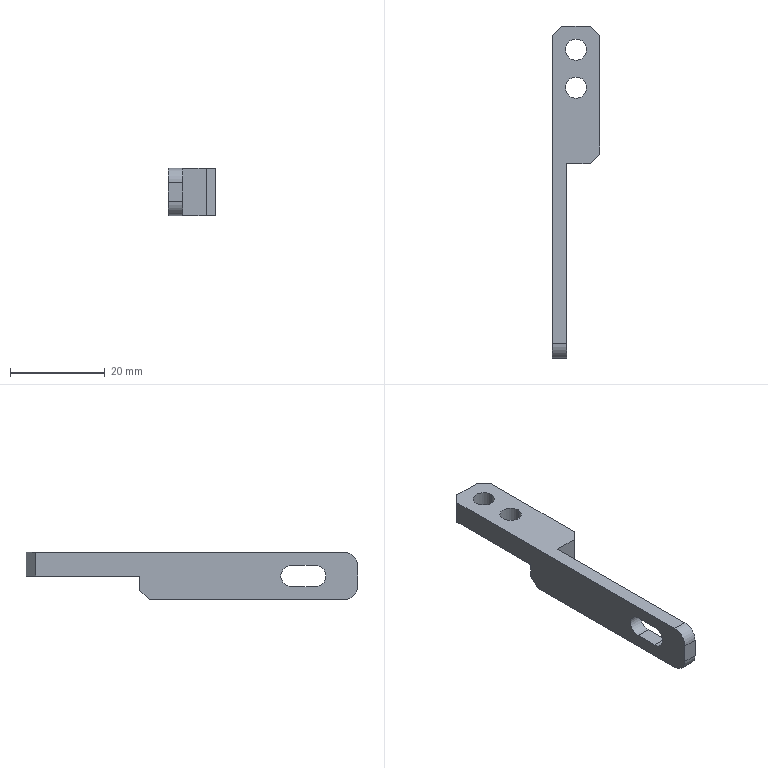Part | SolidWorks | features ICE 3, Chamfer 1, Extrusion 1, Fillet 1, HoleWzd 1 | 1 solid | 24 faces | box 10 x 70 x 10 mm | volume 2584 mm3 | plane 16 | cylinder 8 | commonest cylinder face diameters 4.5 x6 6 x2
STEP:
#1=CARTESIAN_POINT('',(-2.25,30.,0.));
#2=VERTEX_POINT('',#1);
#3=CARTESIAN_POINT('',(2.25,30.,0.));
#4=VERTEX_POINT('',#3);
#5=CARTESIAN_POINT('',(0.,30.,0.));
#6=DIRECTION('',(0.,0.,1.));
#7=DIRECTION('',(0.,-1.,0.));
#8=AXIS2_PLACEMENT_3D('',#5,#6,#7);
#9=CIRCLE('',#8,2.25);
#10=EDGE_CURVE('',#2,#4,#9,.T.);
#11=ORIENTED_EDGE('',*,*,#10,.F.);
#12=CARTESIAN_POINT('',(-2.25,30.,5.));
#13=VERTEX_POINT('',#12);
#14=CARTESIAN_POINT('',(-2.25,30.,5.));
#15=DIRECTION('',(0.,0.,1.));
#16=VECTOR('',#15,1000.);
#17=LINE('',#14,#16);
#18=EDGE_CURVE('',#2,#13,#17,.T.);
#19=ORIENTED_EDGE('',*,*,#18,.T.);
#20=CARTESIAN_POINT('',(2.25,30.,5.));
#21=VERTEX_POINT('',#20);
#22=CARTESIAN_POINT('',(0.,30.,5.));
#23=DIRECTION('',(0.,0.,1.));
#24=DIRECTION('',(1.,0.,0.));
#25=AXIS2_PLACEMENT_3D('',#22,#23,#24);
#26=CIRCLE('',#25,2.25);
#27=EDGE_CURVE('',#13,#21,#26,.T.);
#28=ORIENTED_EDGE('',*,*,#27,.T.);
#29=CARTESIAN_POINT('',(2.25,30.,5.));
#30=DIRECTION('',(0.,0.,1.));
#31=VECTOR('',#30,1000.);
#32=LINE('',#29,#31);
#33=EDGE_CURVE('',#4,#21,#32,.T.);
#34=ORIENTED_EDGE('',*,*,#33,.F.);
#35=EDGE_LOOP('',(#11,#19,#28,#34));
#36=FACE_OUTER_BOUND('',#35,.T.);
#37=CARTESIAN_POINT('',(0.,30.,5.));
#38=DIRECTION('',(0.,0.,1.));
#39=DIRECTION('',(1.,0.,0.));
#40=AXIS2_PLACEMENT_3D('',#37,#38,#39);
#41=CYLINDRICAL_SURFACE('',#40,2.25);
#42=ADVANCED_FACE('',(#36),#41,.F.);
#43=CARTESIAN_POINT('',(-2.25,22.,0.));
#44=VERTEX_POINT('',#43);
#45=CARTESIAN_POINT('',(2.25,22.,0.));
#46=VERTEX_POINT('',#45);
#47=CARTESIAN_POINT('',(0.,22.,0.));
#48=DIRECTION('',(0.,0.,1.));
#49=DIRECTION('',(0.,-1.,0.));
#50=AXIS2_PLACEMENT_3D('',#47,#48,#49);
#51=CIRCLE('',#50,2.25);
#52=EDGE_CURVE('',#44,#46,#51,.T.);
#53=ORIENTED_EDGE('',*,*,#52,.F.);
#54=CARTESIAN_POINT('',(-2.25,22.,5.));
#55=VERTEX_POINT('',#54);
#56=CARTESIAN_POINT('',(-2.25,22.,5.));
#57=DIRECTION('',(0.,0.,1.));
#58=VECTOR('',#57,1000.);
#59=LINE('',#56,#58);
#60=EDGE_CURVE('',#44,#55,#59,.T.);
#61=ORIENTED_EDGE('',*,*,#60,.T.);
#62=CARTESIAN_POINT('',(2.25,22.,5.));
#63=VERTEX_POINT('',#62);
#64=CARTESIAN_POINT('',(0.,22.,5.));
#65=DIRECTION('',(0.,0.,1.));
#66=DIRECTION('',(1.,0.,0.));
#67=AXIS2_PLACEMENT_3D('',#64,#65,#66);
#68=CIRCLE('',#67,2.25);
#69=EDGE_CURVE('',#55,#63,#68,.T.);
#70=ORIENTED_EDGE('',*,*,#69,.T.);
#71=CARTESIAN_POINT('',(2.25,22.,5.));
#72=DIRECTION('',(0.,0.,1.));
#73=VECTOR('',#72,1000.);
#74=LINE('',#71,#73);
#75=EDGE_CURVE('',#46,#63,#74,.T.);
#76=ORIENTED_EDGE('',*,*,#75,.F.);
#77=EDGE_LOOP('',(#53,#61,#70,#76));
#78=FACE_OUTER_BOUND('',#77,.T.);
#79=CARTESIAN_POINT('',(0.,22.,5.));
#80=DIRECTION('',(0.,0.,1.));
#81=DIRECTION('',(1.,0.,0.));
#82=AXIS2_PLACEMENT_3D('',#79,#80,#81);
#83=CYLINDRICAL_SURFACE('',#82,2.25);
#84=ADVANCED_FACE('',(#78),#83,.F.);
#85=CARTESIAN_POINT('',(5.,8.,5.));
#86=VERTEX_POINT('',#85);
#87=CARTESIAN_POINT('',(5.,33.,5.));
#88=VERTEX_POINT('',#87);
#89=CARTESIAN_POINT('',(5.,-35.,5.));
#90=DIRECTION('',(0.,1.,0.));
#91=VECTOR('',#90,1000.);
#92=LINE('',#89,#91);
#93=EDGE_CURVE('',#86,#88,#92,.T.);
#94=ORIENTED_EDGE('',*,*,#93,.F.);
#95=CARTESIAN_POINT('',(5.,8.,-5.));
#96=VERTEX_POINT('',#95);
#97=CARTESIAN_POINT('',(5.,8.,5.));
#98=DIRECTION('',(0.,0.,-1.));
#99=VECTOR('',#98,1000.);
#100=LINE('',#97,#99);
#101=EDGE_CURVE('',#86,#96,#100,.T.);
#102=ORIENTED_EDGE('',*,*,#101,.T.);
#103=CARTESIAN_POINT('',(5.,9.,-5.));
#104=VERTEX_POINT('',#103);
#105=CARTESIAN_POINT('',(5.,-35.,-5.));
#106=DIRECTION('',(0.,1.,0.));
#107=VECTOR('',#106,1000.);
#108=LINE('',#105,#107);
#109=EDGE_CURVE('',#96,#104,#108,.T.);
#110=ORIENTED_EDGE('',*,*,#109,.T.);
#111=CARTESIAN_POINT('',(5.,11.,-3.));
#112=VERTEX_POINT('',#111);
#113=CARTESIAN_POINT('',(5.,9.,-5.));
#114=DIRECTION('',(0.,0.7071,0.7071));
#115=VECTOR('',#114,1000.);
#116=LINE('',#113,#115);
#117=EDGE_CURVE('',#104,#112,#116,.T.);
#118=ORIENTED_EDGE('',*,*,#117,.T.);
#119=CARTESIAN_POINT('',(5.,11.,0.));
#120=VERTEX_POINT('',#119);
#121=CARTESIAN_POINT('',(5.,11.,-5.));
#122=DIRECTION('',(0.,0.,-1.));
#123=VECTOR('',#122,1000.);
#124=LINE('',#121,#123);
#125=EDGE_CURVE('',#120,#112,#124,.T.);
#126=ORIENTED_EDGE('',*,*,#125,.F.);
#127=CARTESIAN_POINT('',(5.,33.,0.));
#128=VERTEX_POINT('',#127);
#129=CARTESIAN_POINT('',(5.,35.,0.));
#130=DIRECTION('',(0.,-1.,0.));
#131=VECTOR('',#130,1000.);
#132=LINE('',#129,#131);
#133=EDGE_CURVE('',#128,#120,#132,.T.);
#134=ORIENTED_EDGE('',*,*,#133,.F.);
#135=CARTESIAN_POINT('',(5.,33.,5.));
#136=DIRECTION('',(0.,0.,1.));
#137=VECTOR('',#136,1000.);
#138=LINE('',#135,#137);
#139=EDGE_CURVE('',#128,#88,#138,.T.);
#140=ORIENTED_EDGE('',*,*,#139,.T.);
#141=EDGE_LOOP('',(#94,#102,#110,#118,#126,#134,#140));
#142=FACE_OUTER_BOUND('',#141,.T.);
#143=CARTESIAN_POINT('',(5.,-35.,5.));
#144=DIRECTION('',(-1.,0.,0.));
#145=DIRECTION('',(0.,0.,1.));
#146=AXIS2_PLACEMENT_3D('',#143,#144,#145);
#147=PLANE('',#146);
#148=ADVANCED_FACE('',(#142),#147,.F.);
#149=CARTESIAN_POINT('',(-3.,35.,0.));
#150=VERTEX_POINT('',#149);
#151=CARTESIAN_POINT('',(3.,35.,0.));
#152=VERTEX_POINT('',#151);
#153=CARTESIAN_POINT('',(-5.,35.,0.));
#154=DIRECTION('',(1.,0.,0.));
#155=VECTOR('',#154,1000.);
#156=LINE('',#153,#155);
#157=EDGE_CURVE('',#150,#152,#156,.T.);
#158=ORIENTED_EDGE('',*,*,#157,.F.);
#159=CARTESIAN_POINT('',(-3.,35.,5.));
#160=VERTEX_POINT('',#159);
#161=CARTESIAN_POINT('',(-3.,35.,5.));
#162=DIRECTION('',(0.,0.,1.));
#163=VECTOR('',#162,1000.);
#164=LINE('',#161,#163);
#165=EDGE_CURVE('',#150,#160,#164,.T.);
#166=ORIENTED_EDGE('',*,*,#165,.T.);
#167=CARTESIAN_POINT('',(3.,35.,5.));
#168=VERTEX_POINT('',#167);
#169=CARTESIAN_POINT('',(-5.,35.,5.));
#170=DIRECTION('',(-1.,0.,0.));
#171=VECTOR('',#170,1000.);
#172=LINE('',#169,#171);
#173=EDGE_CURVE('',#168,#160,#172,.T.);
#174=ORIENTED_EDGE('',*,*,#173,.F.);
#175=CARTESIAN_POINT('',(3.,35.,5.));
#176=DIRECTION('',(0.,0.,-1.));
#177=VECTOR('',#176,1000.);
#178=LINE('',#175,#177);
#179=EDGE_CURVE('',#168,#152,#178,.T.);
#180=ORIENTED_EDGE('',*,*,#179,.T.);
#181=EDGE_LOOP('',(#158,#166,#174,#180));
#182=FACE_OUTER_BOUND('',#181,.T.);
#183=CARTESIAN_POINT('',(-5.,35.,5.));
#184=DIRECTION('',(0.,-1.,0.));
#185=DIRECTION('',(0.,0.,-1.));
#186=AXIS2_PLACEMENT_3D('',#183,#184,#185);
#187=PLANE('',#186);
#188=ADVANCED_FACE('',(#182),#187,.F.);
#189=CARTESIAN_POINT('',(-5.,-21.,-2.25));
#190=VERTEX_POINT('',#189);
#191=CARTESIAN_POINT('',(-5.,-26.,-2.25));
#192=VERTEX_POINT('',#191);
#193=CARTESIAN_POINT('',(-5.,-21.,-2.25));
#194=DIRECTION('',(0.,-1.,0.));
#195=VECTOR('',#194,1000.);
#196=LINE('',#193,#195);
#197=EDGE_CURVE('',#190,#192,#196,.T.);
#198=ORIENTED_EDGE('',*,*,#197,.F.);
#199=CARTESIAN_POINT('',(-5.,-21.,2.25));
#200=VERTEX_POINT('',#199);
#201=CARTESIAN_POINT('',(-5.,-21.,0.));
#202=DIRECTION('',(-1.,0.,0.));
#203=DIRECTION('',(0.,0.,1.));
#204=AXIS2_PLACEMENT_3D('',#201,#202,#203);
#205=CIRCLE('',#204,2.25);
#206=EDGE_CURVE('',#200,#190,#205,.T.);
#207=ORIENTED_EDGE('',*,*,#206,.F.);
#208=CARTESIAN_POINT('',(-5.,-26.,2.25));
#209=VERTEX_POINT('',#208);
#210=CARTESIAN_POINT('',(-5.,-21.,2.25));
#211=DIRECTION('',(0.,1.,0.));
#212=VECTOR('',#211,1000.);
#213=LINE('',#210,#212);
#214=EDGE_CURVE('',#209,#200,#213,.T.);
#215=ORIENTED_EDGE('',*,*,#214,.F.);
#216=CARTESIAN_POINT('',(-5.,-26.,0.));
#217=DIRECTION('',(-1.,0.,0.));
#218=DIRECTION('',(0.,0.,1.));
#219=AXIS2_PLACEMENT_3D('',#216,#217,#218);
#220=CIRCLE('',#219,2.25);
#221=EDGE_CURVE('',#192,#209,#220,.T.);
#222=ORIENTED_EDGE('',*,*,#221,.F.);
#223=EDGE_LOOP('',(#198,#207,#215,#222));
#224=FACE_BOUND('',#223,.T.);
#225=CARTESIAN_POINT('',(-5.,11.,0.));
#226=VERTEX_POINT('',#225);
#227=CARTESIAN_POINT('',(-5.,11.,-3.));
#228=VERTEX_POINT('',#227);
#229=CARTESIAN_POINT('',(-5.,11.,-5.));
#230=DIRECTION('',(0.,0.,-1.));
#231=VECTOR('',#230,1000.);
#232=LINE('',#229,#231);
#233=EDGE_CURVE('',#226,#228,#232,.T.);
#234=ORIENTED_EDGE('',*,*,#233,.T.);
#235=CARTESIAN_POINT('',(-5.,9.,-5.));
#236=VERTEX_POINT('',#235);
#237=CARTESIAN_POINT('',(-5.,9.,-5.));
#238=DIRECTION('',(0.,-0.7071,-0.7071));
#239=VECTOR('',#238,1000.);
#240=LINE('',#237,#239);
#241=EDGE_CURVE('',#228,#236,#240,.T.);
#242=ORIENTED_EDGE('',*,*,#241,.T.);
#243=CARTESIAN_POINT('',(-5.,-32.,-5.));
#244=VERTEX_POINT('',#243);
#245=CARTESIAN_POINT('',(-5.,-35.,-5.));
#246=DIRECTION('',(0.,-1.,0.));
#247=VECTOR('',#246,1000.);
#248=LINE('',#245,#247);
#249=EDGE_CURVE('',#236,#244,#248,.T.);
#250=ORIENTED_EDGE('',*,*,#249,.T.);
#251=CARTESIAN_POINT('',(-5.,-35.,-2.));
#252=VERTEX_POINT('',#251);
#253=CARTESIAN_POINT('',(-5.,-32.,-2.));
#254=DIRECTION('',(-1.,0.,0.));
#255=DIRECTION('',(0.,0.,-1.));
#256=AXIS2_PLACEMENT_3D('',#253,#254,#255);
#257=CIRCLE('',#256,3.);
#258=EDGE_CURVE('',#244,#252,#257,.T.);
#259=ORIENTED_EDGE('',*,*,#258,.T.);
#260=CARTESIAN_POINT('',(-5.,-35.,2.));
#261=VERTEX_POINT('',#260);
#262=CARTESIAN_POINT('',(-5.,-35.,5.));
#263=DIRECTION('',(0.,0.,-1.));
#264=VECTOR('',#263,1000.);
#265=LINE('',#262,#264);
#266=EDGE_CURVE('',#261,#252,#265,.T.);
#267=ORIENTED_EDGE('',*,*,#266,.F.);
#268=CARTESIAN_POINT('',(-5.,-32.,5.));
#269=VERTEX_POINT('',#268);
#270=CARTESIAN_POINT('',(-5.,-32.,2.));
#271=DIRECTION('',(-1.,0.,0.));
#272=DIRECTION('',(0.,0.,-1.));
#273=AXIS2_PLACEMENT_3D('',#270,#271,#272);
#274=CIRCLE('',#273,3.);
#275=EDGE_CURVE('',#261,#269,#274,.T.);
#276=ORIENTED_EDGE('',*,*,#275,.T.);
#277=CARTESIAN_POINT('',(-5.,33.,5.));
#278=VERTEX_POINT('',#277);
#279=CARTESIAN_POINT('',(-5.,-35.,5.));
#280=DIRECTION('',(0.,-1.,0.));
#281=VECTOR('',#280,1000.);
#282=LINE('',#279,#281);
#283=EDGE_CURVE('',#278,#269,#282,.T.);
#284=ORIENTED_EDGE('',*,*,#283,.F.);
#285=CARTESIAN_POINT('',(-5.,33.,0.));
#286=VERTEX_POINT('',#285);
#287=CARTESIAN_POINT('',(-5.,33.,5.));
#288=DIRECTION('',(0.,0.,-1.));
#289=VECTOR('',#288,1000.);
#290=LINE('',#287,#289);
#291=EDGE_CURVE('',#278,#286,#290,.T.);
#292=ORIENTED_EDGE('',*,*,#291,.T.);
#293=CARTESIAN_POINT('',(-5.,35.,0.));
#294=DIRECTION('',(0.,-1.,0.));
#295=VECTOR('',#294,1000.);
#296=LINE('',#293,#295);
#297=EDGE_CURVE('',#286,#226,#296,.T.);
#298=ORIENTED_EDGE('',*,*,#297,.T.);
#299=EDGE_LOOP('',(#234,#242,#250,#259,#267,#276,#284,#292,#298));
#300=FACE_OUTER_BOUND('',#299,.T.);
#301=CARTESIAN_POINT('',(-5.,-35.,5.));
#302=DIRECTION('',(1.,0.,0.));
#303=DIRECTION('',(0.,0.,-1.));
#304=AXIS2_PLACEMENT_3D('',#301,#302,#303);
#305=PLANE('',#304);
#306=ADVANCED_FACE('',(#224,#300),#305,.F.);
#307=ORIENTED_EDGE('',*,*,#266,.T.);
#308=CARTESIAN_POINT('',(-2.,-35.,-2.));
#309=VERTEX_POINT('',#308);
#310=CARTESIAN_POINT('',(-2.,-35.,-2.));
#311=DIRECTION('',(1.,0.,0.));
#312=VECTOR('',#311,1000.);
#313=LINE('',#310,#312);
#314=EDGE_CURVE('',#252,#309,#313,.T.);
#315=ORIENTED_EDGE('',*,*,#314,.T.);
#316=CARTESIAN_POINT('',(-2.,-35.,2.));
#317=VERTEX_POINT('',#316);
#318=CARTESIAN_POINT('',(-2.,-35.,-5.));
#319=DIRECTION('',(0.,0.,1.));
#320=VECTOR('',#319,1000.);
#321=LINE('',#318,#320);
#322=EDGE_CURVE('',#309,#317,#321,.T.);
#323=ORIENTED_EDGE('',*,*,#322,.T.);
#324=CARTESIAN_POINT('',(-5.,-35.,2.));
#325=DIRECTION('',(-1.,0.,0.));
#326=VECTOR('',#325,1000.);
#327=LINE('',#324,#326);
#328=EDGE_CURVE('',#317,#261,#327,.T.);
#329=ORIENTED_EDGE('',*,*,#328,.T.);
#330=EDGE_LOOP('',(#307,#315,#323,#329));
#331=FACE_OUTER_BOUND('',#330,.T.);
#332=CARTESIAN_POINT('',(-5.,-35.,5.));
#333=DIRECTION('',(0.,1.,0.));
#334=DIRECTION('',(0.,0.,1.));
#335=AXIS2_PLACEMENT_3D('',#332,#333,#334);
#336=PLANE('',#335);
#337=ADVANCED_FACE('',(#331),#336,.F.);
#338=CARTESIAN_POINT('',(0.,30.,5.));
#339=DIRECTION('',(0.,0.,1.));
#340=DIRECTION('',(1.,0.,0.));
#341=AXIS2_PLACEMENT_3D('',#338,#339,#340);
#342=CIRCLE('',#341,2.25);
#343=EDGE_CURVE('',#21,#13,#342,.T.);
#344=ORIENTED_EDGE('',*,*,#343,.F.);
#345=ORIENTED_EDGE('',*,*,#27,.F.);
#346=EDGE_LOOP('',(#344,#345));
#347=FACE_BOUND('',#346,.T.);
#348=CARTESIAN_POINT('',(0.,22.,5.));
#349=DIRECTION('',(0.,0.,1.));
#350=DIRECTION('',(1.,0.,0.));
#351=AXIS2_PLACEMENT_3D('',#348,#349,#350);
#352=CIRCLE('',#351,2.25);
#353=EDGE_CURVE('',#63,#55,#352,.T.);
#354=ORIENTED_EDGE('',*,*,#353,.F.);
#355=ORIENTED_EDGE('',*,*,#69,.F.);
#356=EDGE_LOOP('',(#354,#355));
#357=FACE_BOUND('',#356,.T.);
#358=CARTESIAN_POINT('',(3.,6.,5.));
#359=VERTEX_POINT('',#358);
#360=CARTESIAN_POINT('',(-2.,6.,5.));
#361=VERTEX_POINT('',#360);
#362=CARTESIAN_POINT('',(5.,6.,5.));
#363=DIRECTION('',(-1.,0.,0.));
#364=VECTOR('',#363,1000.);
#365=LINE('',#362,#364);
#366=EDGE_CURVE('',#359,#361,#365,.T.);
#367=ORIENTED_EDGE('',*,*,#366,.F.);
#368=CARTESIAN_POINT('',(3.,6.,5.));
#369=DIRECTION('',(0.7071,0.7071,0.));
#370=VECTOR('',#369,1000.);
#371=LINE('',#368,#370);
#372=EDGE_CURVE('',#359,#86,#371,.T.);
#373=ORIENTED_EDGE('',*,*,#372,.T.);
#374=ORIENTED_EDGE('',*,*,#93,.T.);
#375=CARTESIAN_POINT('',(3.,35.,5.));
#376=DIRECTION('',(-0.7071,0.7071,0.));
#377=VECTOR('',#376,1000.);
#378=LINE('',#375,#377);
#379=EDGE_CURVE('',#88,#168,#378,.T.);
#380=ORIENTED_EDGE('',*,*,#379,.T.);
#381=ORIENTED_EDGE('',*,*,#173,.T.);
#382=CARTESIAN_POINT('',(-5.,33.,5.));
#383=DIRECTION('',(-0.7071,-0.7071,0.));
#384=VECTOR('',#383,1000.);
#385=LINE('',#382,#384);
#386=EDGE_CURVE('',#160,#278,#385,.T.);
#387=ORIENTED_EDGE('',*,*,#386,.T.);
#388=ORIENTED_EDGE('',*,*,#283,.T.);
#389=CARTESIAN_POINT('',(-2.,-32.,5.));
#390=VERTEX_POINT('',#389);
#391=CARTESIAN_POINT('',(0.,-32.,5.));
#392=DIRECTION('',(1.,0.,0.));
#393=VECTOR('',#392,1000.);
#394=LINE('',#391,#393);
#395=EDGE_CURVE('',#269,#390,#394,.T.);
#396=ORIENTED_EDGE('',*,*,#395,.T.);
#397=CARTESIAN_POINT('',(-2.,-35.,5.));
#398=DIRECTION('',(0.,-1.,0.));
#399=VECTOR('',#398,1000.);
#400=LINE('',#397,#399);
#401=EDGE_CURVE('',#361,#390,#400,.T.);
#402=ORIENTED_EDGE('',*,*,#401,.F.);
#403=EDGE_LOOP('',(#367,#373,#374,#380,#381,#387,#388,#396,#402));
#404=FACE_OUTER_BOUND('',#403,.T.);
#405=CARTESIAN_POINT('',(0.,0.,5.));
#406=DIRECTION('',(0.,0.,-1.));
#407=DIRECTION('',(-1.,0.,0.));
#408=AXIS2_PLACEMENT_3D('',#405,#406,#407);
#409=PLANE('',#408);
#410=ADVANCED_FACE('',(#347,#357,#404),#409,.F.);
#411=ORIENTED_EDGE('',*,*,#109,.F.);
#412=CARTESIAN_POINT('',(3.,6.,-5.));
#413=VERTEX_POINT('',#412);
#414=CARTESIAN_POINT('',(-1.5,1.5,-5.));
#415=DIRECTION('',(-0.7071,-0.7071,0.));
#416=VECTOR('',#415,1000.);
#417=LINE('',#414,#416);
#418=EDGE_CURVE('',#96,#413,#417,.T.);
#419=ORIENTED_EDGE('',*,*,#418,.T.);
#420=CARTESIAN_POINT('',(-2.,6.,-5.));
#421=VERTEX_POINT('',#420);
#422=CARTESIAN_POINT('',(5.,6.,-5.));
#423=DIRECTION('',(-1.,0.,0.));
#424=VECTOR('',#423,1000.);
#425=LINE('',#422,#424);
#426=EDGE_CURVE('',#413,#421,#425,.T.);
#427=ORIENTED_EDGE('',*,*,#426,.T.);
#428=CARTESIAN_POINT('',(-2.,-32.,-5.));
#429=VERTEX_POINT('',#428);
#430=CARTESIAN_POINT('',(-2.,-35.,-5.));
#431=DIRECTION('',(0.,-1.,0.));
#432=VECTOR('',#431,1000.);
#433=LINE('',#430,#432);
#434=EDGE_CURVE('',#421,#429,#433,.T.);
#435=ORIENTED_EDGE('',*,*,#434,.T.);
#436=CARTESIAN_POINT('',(-5.,-32.,-5.));
#437=DIRECTION('',(-1.,0.,0.));
#438=VECTOR('',#437,1000.);
#439=LINE('',#436,#438);
#440=EDGE_CURVE('',#429,#244,#439,.T.);
#441=ORIENTED_EDGE('',*,*,#440,.T.);
#442=ORIENTED_EDGE('',*,*,#249,.F.);
#443=CARTESIAN_POINT('',(5.,9.,-5.));
#444=DIRECTION('',(1.,0.,0.));
#445=VECTOR('',#444,1000.);
#446=LINE('',#443,#445);
#447=EDGE_CURVE('',#236,#104,#446,.T.);
#448=ORIENTED_EDGE('',*,*,#447,.T.);
#449=EDGE_LOOP('',(#411,#419,#427,#435,#441,#442,#448));
#450=FACE_OUTER_BOUND('',#449,.T.);
#451=CARTESIAN_POINT('',(0.,0.,-5.));
#452=DIRECTION('',(0.,0.,-1.));
#453=DIRECTION('',(-1.,0.,0.));
#454=AXIS2_PLACEMENT_3D('',#451,#452,#453);
#455=PLANE('',#454);
#456=ADVANCED_FACE('',(#450),#455,.T.);
#457=CARTESIAN_POINT('',(-2.,-26.,2.25));
#458=VERTEX_POINT('',#457);
#459=CARTESIAN_POINT('',(-2.,-21.,2.25));
#460=VERTEX_POINT('',#459);
#461=CARTESIAN_POINT('',(-2.,-35.,2.25));
#462=DIRECTION('',(0.,1.,0.));
#463=VECTOR('',#462,1000.);
#464=LINE('',#461,#463);
#465=EDGE_CURVE('',#458,#460,#464,.T.);
#466=ORIENTED_EDGE('',*,*,#465,.T.);
#467=CARTESIAN_POINT('',(-2.,-21.,-2.25));
#468=VERTEX_POINT('',#467);
#469=CARTESIAN_POINT('',(-2.,-21.,0.));
#470=DIRECTION('',(-1.,0.,0.));
#471=DIRECTION('',(0.,0.,1.));
#472=AXIS2_PLACEMENT_3D('',#469,#470,#471);
#473=CIRCLE('',#472,2.25);
#474=EDGE_CURVE('',#460,#468,#473,.T.);
#475=ORIENTED_EDGE('',*,*,#474,.T.);
#476=CARTESIAN_POINT('',(-2.,-26.,-2.25));
#477=VERTEX_POINT('',#476);
#478=CARTESIAN_POINT('',(-2.,-35.,-2.25));
#479=DIRECTION('',(0.,-1.,0.));
#480=VECTOR('',#479,1000.);
#481=LINE('',#478,#480);
#482=EDGE_CURVE('',#468,#477,#481,.T.);
#483=ORIENTED_EDGE('',*,*,#482,.T.);
#484=CARTESIAN_POINT('',(-2.,-26.,0.));
#485=DIRECTION('',(-1.,0.,0.));
#486=DIRECTION('',(0.,0.,1.));
#487=AXIS2_PLACEMENT_3D('',#484,#485,#486);
#488=CIRCLE('',#487,2.25);
#489=EDGE_CURVE('',#477,#458,#488,.T.);
#490=ORIENTED_EDGE('',*,*,#489,.T.);
#491=EDGE_LOOP('',(#466,#475,#483,#490));
#492=FACE_BOUND('',#491,.T.);
#493=ORIENTED_EDGE('',*,*,#322,.F.);
#494=CARTESIAN_POINT('',(-2.,-32.,-2.));
#495=DIRECTION('',(1.,0.,0.));
#496=DIRECTION('',(0.,0.,1.));
#497=AXIS2_PLACEMENT_3D('',#494,#495,#496);
#498=CIRCLE('',#497,3.);
#499=EDGE_CURVE('',#309,#429,#498,.T.);
#500=ORIENTED_EDGE('',*,*,#499,.T.);
#501=ORIENTED_EDGE('',*,*,#434,.F.);
#502=CARTESIAN_POINT('',(-2.,6.,-5.));
#503=DIRECTION('',(0.,0.,1.));
#504=VECTOR('',#503,1000.);
#505=LINE('',#502,#504);
#506=EDGE_CURVE('',#421,#361,#505,.T.);
#507=ORIENTED_EDGE('',*,*,#506,.T.);
#508=ORIENTED_EDGE('',*,*,#401,.T.);
#509=CARTESIAN_POINT('',(-2.,-32.,2.));
#510=DIRECTION('',(1.,0.,0.));
#511=DIRECTION('',(0.,0.,1.));
#512=AXIS2_PLACEMENT_3D('',#509,#510,#511);
#513=CIRCLE('',#512,3.);
#514=EDGE_CURVE('',#390,#317,#513,.T.);
#515=ORIENTED_EDGE('',*,*,#514,.T.);
#516=EDGE_LOOP('',(#493,#500,#501,#507,#508,#515));
#517=FACE_OUTER_BOUND('',#516,.T.);
#518=CARTESIAN_POINT('',(-2.,-35.,-5.));
#519=DIRECTION('',(-1.,0.,0.));
#520=DIRECTION('',(0.,0.,1.));
#521=AXIS2_PLACEMENT_3D('',#518,#519,#520);
#522=PLANE('',#521);
#523=ADVANCED_FACE('',(#492,#517),#522,.F.);
#524=ORIENTED_EDGE('',*,*,#426,.F.);
#525=CARTESIAN_POINT('',(3.,6.,-5.));
#526=DIRECTION('',(0.,0.,1.));
#527=VECTOR('',#526,1000.);
#528=LINE('',#525,#527);
#529=EDGE_CURVE('',#413,#359,#528,.T.);
#530=ORIENTED_EDGE('',*,*,#529,.T.);
#531=ORIENTED_EDGE('',*,*,#366,.T.);
#532=ORIENTED_EDGE('',*,*,#506,.F.);
#533=EDGE_LOOP('',(#524,#530,#531,#532));
#534=FACE_OUTER_BOUND('',#533,.T.);
#535=CARTESIAN_POINT('',(5.,6.,-5.));
#536=DIRECTION('',(0.,1.,0.));
#537=DIRECTION('',(0.,0.,1.));
#538=AXIS2_PLACEMENT_3D('',#535,#536,#537);
#539=PLANE('',#538);
#540=ADVANCED_FACE('',(#534),#539,.F.);
#541=ORIENTED_EDGE('',*,*,#125,.T.);
#542=CARTESIAN_POINT('',(-5.,11.,-3.));
#543=DIRECTION('',(-1.,0.,0.));
#544=VECTOR('',#543,1000.);
#545=LINE('',#542,#544);
#546=EDGE_CURVE('',#112,#228,#545,.T.);
#547=ORIENTED_EDGE('',*,*,#546,.T.);
#548=ORIENTED_EDGE('',*,*,#233,.F.);
#549=CARTESIAN_POINT('',(-5.,11.,0.));
#550=DIRECTION('',(1.,0.,0.));
#551=VECTOR('',#550,1000.);
#552=LINE('',#549,#551);
#553=EDGE_CURVE('',#226,#120,#552,.T.);
#554=ORIENTED_EDGE('',*,*,#553,.T.);
#555=EDGE_LOOP('',(#541,#547,#548,#554));
#556=FACE_OUTER_BOUND('',#555,.T.);
#557=CARTESIAN_POINT('',(-5.,11.,-5.));
#558=DIRECTION('',(0.,-1.,0.));
#559=DIRECTION('',(0.,0.,-1.));
#560=AXIS2_PLACEMENT_3D('',#557,#558,#559);
#561=PLANE('',#560);
#562=ADVANCED_FACE('',(#556),#561,.F.);
#563=CARTESIAN_POINT('',(0.,30.,0.));
#564=DIRECTION('',(0.,0.,1.));
#565=DIRECTION('',(0.,-1.,0.));
#566=AXIS2_PLACEMENT_3D('',#563,#564,#565);
#567=CIRCLE('',#566,2.25);
#568=EDGE_CURVE('',#4,#2,#567,.T.);
#569=ORIENTED_EDGE('',*,*,#568,.T.);
#570=ORIENTED_EDGE('',*,*,#10,.T.);
#571=EDGE_LOOP('',(#569,#570));
#572=FACE_BOUND('',#571,.T.);
#573=CARTESIAN_POINT('',(0.,22.,0.));
#574=DIRECTION('',(0.,0.,1.));
#575=DIRECTION('',(0.,-1.,0.));
#576=AXIS2_PLACEMENT_3D('',#573,#574,#575);
#577=CIRCLE('',#576,2.25);
#578=EDGE_CURVE('',#46,#44,#577,.T.);
#579=ORIENTED_EDGE('',*,*,#578,.T.);
#580=ORIENTED_EDGE('',*,*,#52,.T.);
#581=EDGE_LOOP('',(#579,#580));
#582=FACE_BOUND('',#581,.T.);
#583=ORIENTED_EDGE('',*,*,#297,.F.);
#584=CARTESIAN_POINT('',(-5.,33.,0.));
#585=DIRECTION('',(0.7071,0.7071,0.));
#586=VECTOR('',#585,1000.);
#587=LINE('',#584,#586);
#588=EDGE_CURVE('',#286,#150,#587,.T.);
#589=ORIENTED_EDGE('',*,*,#588,.T.);
#590=ORIENTED_EDGE('',*,*,#157,.T.);
#591=CARTESIAN_POINT('',(3.,35.,0.));
#592=DIRECTION('',(0.7071,-0.7071,0.));
#593=VECTOR('',#592,1000.);
#594=LINE('',#591,#593);
#595=EDGE_CURVE('',#152,#128,#594,.T.);
#596=ORIENTED_EDGE('',*,*,#595,.T.);
#597=ORIENTED_EDGE('',*,*,#133,.T.);
#598=ORIENTED_EDGE('',*,*,#553,.F.);
#599=EDGE_LOOP('',(#583,#589,#590,#596,#597,#598));
#600=FACE_OUTER_BOUND('',#599,.T.);
#601=CARTESIAN_POINT('',(-5.,35.,0.));
#602=DIRECTION('',(0.,0.,1.));
#603=DIRECTION('',(0.,-1.,0.));
#604=AXIS2_PLACEMENT_3D('',#601,#602,#603);
#605=PLANE('',#604);
#606=ADVANCED_FACE('',(#572,#582,#600),#605,.F.);
#607=CARTESIAN_POINT('',(5.,-21.,2.25));
#608=DIRECTION('',(-1.,0.,0.));
#609=VECTOR('',#608,1000.);
#610=LINE('',#607,#609);
#611=EDGE_CURVE('',#460,#200,#610,.T.);
#612=ORIENTED_EDGE('',*,*,#611,.T.);
#613=ORIENTED_EDGE('',*,*,#206,.T.);
#614=CARTESIAN_POINT('',(5.,-21.,-2.25));
#615=DIRECTION('',(-1.,0.,0.));
#616=VECTOR('',#615,1000.);
#617=LINE('',#614,#616);
#618=EDGE_CURVE('',#468,#190,#617,.T.);
#619=ORIENTED_EDGE('',*,*,#618,.F.);
#620=ORIENTED_EDGE('',*,*,#474,.F.);
#621=EDGE_LOOP('',(#612,#613,#619,#620));
#622=FACE_OUTER_BOUND('',#621,.T.);
#623=CARTESIAN_POINT('',(5.,-21.,0.));
#624=DIRECTION('',(-1.,0.,0.));
#625=DIRECTION('',(0.,0.,1.));
#626=AXIS2_PLACEMENT_3D('',#623,#624,#625);
#627=CYLINDRICAL_SURFACE('',#626,2.25);
#628=ADVANCED_FACE('',(#622),#627,.F.);
#629=CARTESIAN_POINT('',(5.,-26.,2.25));
#630=DIRECTION('',(-1.,0.,0.));
#631=VECTOR('',#630,1000.);
#632=LINE('',#629,#631);
#633=EDGE_CURVE('',#458,#209,#632,.T.);
#634=ORIENTED_EDGE('',*,*,#633,.T.);
#635=ORIENTED_EDGE('',*,*,#214,.T.);
#636=ORIENTED_EDGE('',*,*,#611,.F.);
#637=ORIENTED_EDGE('',*,*,#465,.F.);
#638=EDGE_LOOP('',(#634,#635,#636,#637));
#639=FACE_OUTER_BOUND('',#638,.T.);
#640=CARTESIAN_POINT('',(5.,-21.,2.25));
#641=DIRECTION('',(0.,0.,1.));
#642=DIRECTION('',(0.,-1.,0.));
#643=AXIS2_PLACEMENT_3D('',#640,#641,#642);
#644=PLANE('',#643);
#645=ADVANCED_FACE('',(#639),#644,.F.);
#646=CARTESIAN_POINT('',(5.,-26.,-2.25));
#647=DIRECTION('',(-1.,0.,0.));
#648=VECTOR('',#647,1000.);
#649=LINE('',#646,#648);
#650=EDGE_CURVE('',#477,#192,#649,.T.);
#651=ORIENTED_EDGE('',*,*,#650,.T.);
#652=ORIENTED_EDGE('',*,*,#221,.T.);
#653=ORIENTED_EDGE('',*,*,#633,.F.);
#654=ORIENTED_EDGE('',*,*,#489,.F.);
#655=EDGE_LOOP('',(#651,#652,#653,#654));
#656=FACE_OUTER_BOUND('',#655,.T.);
#657=CARTESIAN_POINT('',(5.,-26.,0.));
#658=DIRECTION('',(-1.,0.,0.));
#659=DIRECTION('',(0.,0.,1.));
#660=AXIS2_PLACEMENT_3D('',#657,#658,#659);
#661=CYLINDRICAL_SURFACE('',#660,2.25);
#662=ADVANCED_FACE('',(#656),#661,.F.);
#663=ORIENTED_EDGE('',*,*,#618,.T.);
#664=ORIENTED_EDGE('',*,*,#197,.T.);
#665=ORIENTED_EDGE('',*,*,#650,.F.);
#666=ORIENTED_EDGE('',*,*,#482,.F.);
#667=EDGE_LOOP('',(#663,#664,#665,#666));
#668=FACE_OUTER_BOUND('',#667,.T.);
#669=CARTESIAN_POINT('',(5.,-21.,-2.25));
#670=DIRECTION('',(0.,0.,-1.));
#671=DIRECTION('',(0.,1.,0.));
#672=AXIS2_PLACEMENT_3D('',#669,#670,#671);
#673=PLANE('',#672);
#674=ADVANCED_FACE('',(#668),#673,.F.);
#675=ORIENTED_EDGE('',*,*,#258,.F.);
#676=ORIENTED_EDGE('',*,*,#440,.F.);
#677=ORIENTED_EDGE('',*,*,#499,.F.);
#678=ORIENTED_EDGE('',*,*,#314,.F.);
#679=EDGE_LOOP('',(#675,#676,#677,#678));
#680=FACE_OUTER_BOUND('',#679,.T.);
#681=CARTESIAN_POINT('',(-5.,-32.,-2.));
#682=DIRECTION('',(-1.,0.,0.));
#683=DIRECTION('',(0.,0.,1.));
#684=AXIS2_PLACEMENT_3D('',#681,#682,#683);
#685=CYLINDRICAL_SURFACE('',#684,3.);
#686=ADVANCED_FACE('',(#680),#685,.T.);
#687=ORIENTED_EDGE('',*,*,#275,.F.);
#688=ORIENTED_EDGE('',*,*,#328,.F.);
#689=ORIENTED_EDGE('',*,*,#514,.F.);
#690=ORIENTED_EDGE('',*,*,#395,.F.);
#691=EDGE_LOOP('',(#687,#688,#689,#690));
#692=FACE_OUTER_BOUND('',#691,.T.);
#693=CARTESIAN_POINT('',(0.,-32.,2.));
#694=DIRECTION('',(1.,0.,0.));
#695=DIRECTION('',(0.,0.,-1.));
#696=AXIS2_PLACEMENT_3D('',#693,#694,#695);
#697=CYLINDRICAL_SURFACE('',#696,3.);
#698=ADVANCED_FACE('',(#692),#697,.T.);
#699=ORIENTED_EDGE('',*,*,#60,.F.);
#700=ORIENTED_EDGE('',*,*,#578,.F.);
#701=ORIENTED_EDGE('',*,*,#75,.T.);
#702=ORIENTED_EDGE('',*,*,#353,.T.);
#703=EDGE_LOOP('',(#699,#700,#701,#702));
#704=FACE_OUTER_BOUND('',#703,.T.);
#705=CARTESIAN_POINT('',(0.,22.,5.));
#706=DIRECTION('',(0.,0.,1.));
#707=DIRECTION('',(1.,0.,0.));
#708=AXIS2_PLACEMENT_3D('',#705,#706,#707);
#709=CYLINDRICAL_SURFACE('',#708,2.25);
#710=ADVANCED_FACE('',(#704),#709,.F.);
#711=ORIENTED_EDGE('',*,*,#18,.F.);
#712=ORIENTED_EDGE('',*,*,#568,.F.);
#713=ORIENTED_EDGE('',*,*,#33,.T.);
#714=ORIENTED_EDGE('',*,*,#343,.T.);
#715=EDGE_LOOP('',(#711,#712,#713,#714));
#716=FACE_OUTER_BOUND('',#715,.T.);
#717=CARTESIAN_POINT('',(0.,30.,5.));
#718=DIRECTION('',(0.,0.,1.));
#719=DIRECTION('',(1.,0.,0.));
#720=AXIS2_PLACEMENT_3D('',#717,#718,#719);
#721=CYLINDRICAL_SURFACE('',#720,2.25);
#722=ADVANCED_FACE('',(#716),#721,.F.);
#723=ORIENTED_EDGE('',*,*,#418,.F.);
#724=ORIENTED_EDGE('',*,*,#101,.F.);
#725=ORIENTED_EDGE('',*,*,#372,.F.);
#726=ORIENTED_EDGE('',*,*,#529,.F.);
#727=EDGE_LOOP('',(#723,#724,#725,#726));
#728=FACE_OUTER_BOUND('',#727,.T.);
#729=CARTESIAN_POINT('',(3.,6.,-5.));
#730=DIRECTION('',(-0.7071,0.7071,0.));
#731=DIRECTION('',(0.,0.,1.));
#732=AXIS2_PLACEMENT_3D('',#729,#730,#731);
#733=PLANE('',#732);
#734=ADVANCED_FACE('',(#728),#733,.F.);
#735=ORIENTED_EDGE('',*,*,#241,.F.);
#736=ORIENTED_EDGE('',*,*,#546,.F.);
#737=ORIENTED_EDGE('',*,*,#117,.F.);
#738=ORIENTED_EDGE('',*,*,#447,.F.);
#739=EDGE_LOOP('',(#735,#736,#737,#738));
#740=FACE_OUTER_BOUND('',#739,.T.);
#741=CARTESIAN_POINT('',(0.,9.,-5.));
#742=DIRECTION('',(0.,0.7071,-0.7071));
#743=DIRECTION('',(-1.,0.,0.));
#744=AXIS2_PLACEMENT_3D('',#741,#742,#743);
#745=PLANE('',#744);
#746=ADVANCED_FACE('',(#740),#745,.T.);
#747=ORIENTED_EDGE('',*,*,#386,.F.);
#748=ORIENTED_EDGE('',*,*,#165,.F.);
#749=ORIENTED_EDGE('',*,*,#588,.F.);
#750=ORIENTED_EDGE('',*,*,#291,.F.);
#751=EDGE_LOOP('',(#747,#748,#749,#750));
#752=FACE_OUTER_BOUND('',#751,.T.);
#753=CARTESIAN_POINT('',(-5.,33.,5.));
#754=DIRECTION('',(0.7071,-0.7071,0.));
#755=DIRECTION('',(0.,0.,-1.));
#756=AXIS2_PLACEMENT_3D('',#753,#754,#755);
#757=PLANE('',#756);
#758=ADVANCED_FACE('',(#752),#757,.F.);
#759=ORIENTED_EDGE('',*,*,#379,.F.);
#760=ORIENTED_EDGE('',*,*,#139,.F.);
#761=ORIENTED_EDGE('',*,*,#595,.F.);
#762=ORIENTED_EDGE('',*,*,#179,.F.);
#763=EDGE_LOOP('',(#759,#760,#761,#762));
#764=FACE_OUTER_BOUND('',#763,.T.);
#765=CARTESIAN_POINT('',(3.,35.,5.));
#766=DIRECTION('',(-0.7071,-0.7071,0.));
#767=DIRECTION('',(0.,0.,-1.));
#768=AXIS2_PLACEMENT_3D('',#765,#766,#767);
#769=PLANE('',#768);
#770=ADVANCED_FACE('',(#764),#769,.F.);
#771=CLOSED_SHELL('',(#42,#84,#148,#188,#306,#337,#410,#456,#523,#540,#562,#606,#628,#645,#662,#674,#686,#698,#710,#722,#734,#746,#758,#770));
#772=MANIFOLD_SOLID_BREP('',#771);
#773=CARTESIAN_POINT('',(0.,0.,0.));
#774=DIRECTION('',(0.,0.,1.));
#775=DIRECTION('',(1.,0.,0.));
#776=AXIS2_PLACEMENT_3D('',#773,#774,#775);
#777=(LENGTH_UNIT()NAMED_UNIT(*)SI_UNIT(.MILLI.,.METRE.));
#778=UNCERTAINTY_MEASURE_WITH_UNIT(LENGTH_MEASURE(0.00001),#777,'','');
#779=(NAMED_UNIT(*)PLANE_ANGLE_UNIT()SI_UNIT($,.RADIAN.));
#780=(NAMED_UNIT(*)SI_UNIT($,.STERADIAN.)SOLID_ANGLE_UNIT());
#781=(GEOMETRIC_REPRESENTATION_CONTEXT(3)GLOBAL_UNCERTAINTY_ASSIGNED_CONTEXT((#778))GLOBAL_UNIT_ASSIGNED_CONTEXT((#777,#779,#780))REPRESENTATION_CONTEXT('',''));
#782=ADVANCED_BREP_SHAPE_REPRESENTATION('',(#772,#776),#781);